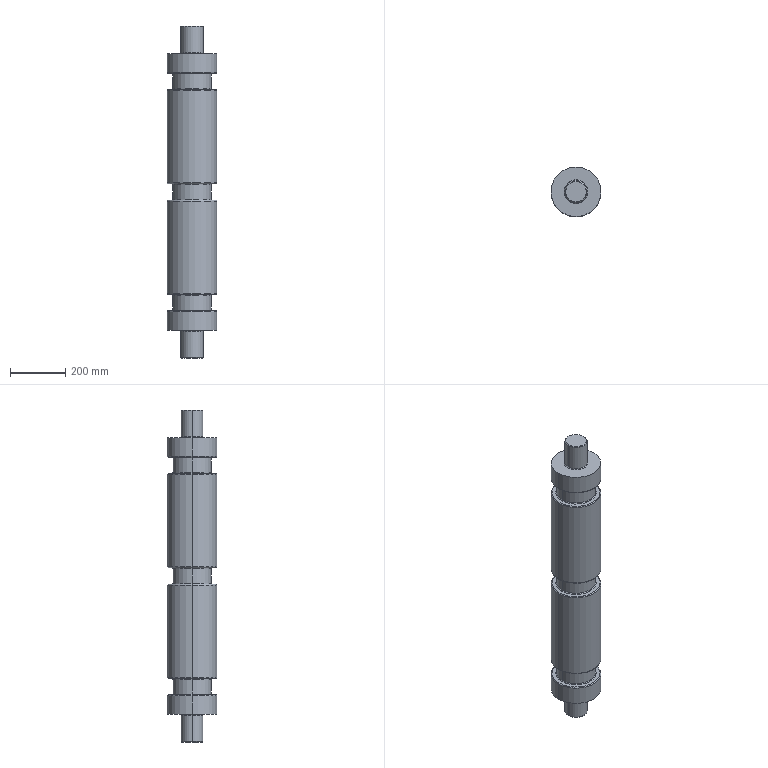Part | SolidWorks | features Chamfer 2, ICE 2, Extrusion 1, Fillet 1, LPattern 1, RefAxis 1, RevCut 1 | 1 solid | 60 faces | box 180 x 180 x 1200 mm | volume 24641407 mm3 | torus 24 | cylinder 18 | plane 10 | cone 8 | commonest cylinder face diameters 180 x8 140 x6 80 x4
STEP:
#1=CARTESIAN_POINT('',(-37.,0.,-100.));
#2=VERTEX_POINT('',#1);
#3=CARTESIAN_POINT('',(37.,0.,-100.));
#4=VERTEX_POINT('',#3);
#5=CARTESIAN_POINT('',(0.,0.,-100.));
#6=DIRECTION('',(0.,0.,-1.));
#7=DIRECTION('',(-1.,0.,0.));
#8=AXIS2_PLACEMENT_3D('',#5,#6,#7);
#9=CIRCLE('',#8,37.);
#10=EDGE_CURVE('',#2,#4,#9,.T.);
#11=ORIENTED_EDGE('',*,*,#10,.F.);
#12=CARTESIAN_POINT('',(-40.,0.,-97.));
#13=VERTEX_POINT('',#12);
#14=CARTESIAN_POINT('',(-37.,0.,-100.));
#15=DIRECTION('',(-0.7071,0.,0.7071));
#16=VECTOR('',#15,1000.);
#17=LINE('',#14,#16);
#18=EDGE_CURVE('',#2,#13,#17,.T.);
#19=ORIENTED_EDGE('',*,*,#18,.T.);
#20=CARTESIAN_POINT('',(40.,0.,-97.));
#21=VERTEX_POINT('',#20);
#22=CARTESIAN_POINT('',(0.,0.,-97.));
#23=DIRECTION('',(0.,0.,1.));
#24=DIRECTION('',(-1.,0.,0.));
#25=AXIS2_PLACEMENT_3D('',#22,#23,#24);
#26=CIRCLE('',#25,40.);
#27=EDGE_CURVE('',#21,#13,#26,.T.);
#28=ORIENTED_EDGE('',*,*,#27,.F.);
#29=CARTESIAN_POINT('',(37.,0.,-100.));
#30=DIRECTION('',(0.7071,0.,0.7071));
#31=VECTOR('',#30,1000.);
#32=LINE('',#29,#31);
#33=EDGE_CURVE('',#4,#21,#32,.T.);
#34=ORIENTED_EDGE('',*,*,#33,.F.);
#35=EDGE_LOOP('',(#11,#19,#28,#34));
#36=FACE_OUTER_BOUND('',#35,.T.);
#37=CARTESIAN_POINT('',(0.,0.,-100.));
#38=DIRECTION('',(0.,0.,1.));
#39=DIRECTION('',(1.,0.,0.));
#40=AXIS2_PLACEMENT_3D('',#37,#38,#39);
#41=CONICAL_SURFACE('',#40,37.,0.7854);
#42=ADVANCED_FACE('',(#36),#41,.T.);
#43=CARTESIAN_POINT('',(-40.,0.,-3.));
#44=VERTEX_POINT('',#43);
#45=CARTESIAN_POINT('',(40.,0.,-3.));
#46=VERTEX_POINT('',#45);
#47=CARTESIAN_POINT('',(0.,0.,-3.));
#48=DIRECTION('',(0.,0.,-1.));
#49=DIRECTION('',(1.,0.,0.));
#50=AXIS2_PLACEMENT_3D('',#47,#48,#49);
#51=CIRCLE('',#50,40.);
#52=EDGE_CURVE('',#44,#46,#51,.T.);
#53=ORIENTED_EDGE('',*,*,#52,.F.);
#54=CARTESIAN_POINT('',(-43.,0.,0.));
#55=VERTEX_POINT('',#54);
#56=CARTESIAN_POINT('',(-40.,0.,-3.));
#57=DIRECTION('',(-0.7071,0.,0.7071));
#58=VECTOR('',#57,1000.);
#59=LINE('',#56,#58);
#60=EDGE_CURVE('',#44,#55,#59,.T.);
#61=ORIENTED_EDGE('',*,*,#60,.T.);
#62=CARTESIAN_POINT('',(43.,0.,0.));
#63=VERTEX_POINT('',#62);
#64=CARTESIAN_POINT('',(0.,0.,0.));
#65=DIRECTION('',(0.,0.,1.));
#66=DIRECTION('',(1.,0.,0.));
#67=AXIS2_PLACEMENT_3D('',#64,#65,#66);
#68=CIRCLE('',#67,43.);
#69=EDGE_CURVE('',#63,#55,#68,.T.);
#70=ORIENTED_EDGE('',*,*,#69,.F.);
#71=CARTESIAN_POINT('',(40.,0.,-3.));
#72=DIRECTION('',(0.7071,0.,0.7071));
#73=VECTOR('',#72,1000.);
#74=LINE('',#71,#73);
#75=EDGE_CURVE('',#46,#63,#74,.T.);
#76=ORIENTED_EDGE('',*,*,#75,.F.);
#77=EDGE_LOOP('',(#53,#61,#70,#76));
#78=FACE_OUTER_BOUND('',#77,.T.);
#79=CARTESIAN_POINT('',(0.,0.,-3.));
#80=DIRECTION('',(0.,0.,1.));
#81=DIRECTION('',(1.,0.,0.));
#82=AXIS2_PLACEMENT_3D('',#79,#80,#81);
#83=CONICAL_SURFACE('',#82,40.,0.7854);
#84=ADVANCED_FACE('',(#78),#83,.T.);
#85=ORIENTED_EDGE('',*,*,#27,.T.);
#86=CARTESIAN_POINT('',(-40.,0.,-100.));
#87=DIRECTION('',(0.,0.,1.));
#88=VECTOR('',#87,1000.);
#89=LINE('',#86,#88);
#90=EDGE_CURVE('',#13,#44,#89,.T.);
#91=ORIENTED_EDGE('',*,*,#90,.T.);
#92=ORIENTED_EDGE('',*,*,#52,.T.);
#93=CARTESIAN_POINT('',(40.,0.,-100.));
#94=DIRECTION('',(0.,0.,1.));
#95=VECTOR('',#94,1000.);
#96=LINE('',#93,#95);
#97=EDGE_CURVE('',#21,#46,#96,.T.);
#98=ORIENTED_EDGE('',*,*,#97,.F.);
#99=EDGE_LOOP('',(#85,#91,#92,#98));
#100=FACE_OUTER_BOUND('',#99,.T.);
#101=CARTESIAN_POINT('',(0.,0.,-100.));
#102=DIRECTION('',(0.,0.,1.));
#103=DIRECTION('',(1.,0.,0.));
#104=AXIS2_PLACEMENT_3D('',#101,#102,#103);
#105=CYLINDRICAL_SURFACE('',#104,40.);
#106=ADVANCED_FACE('',(#100),#105,.T.);
#107=CARTESIAN_POINT('',(37.,0.,1100.));
#108=VERTEX_POINT('',#107);
#109=CARTESIAN_POINT('',(-37.,0.,1100.));
#110=VERTEX_POINT('',#109);
#111=CARTESIAN_POINT('',(0.,0.,1100.));
#112=DIRECTION('',(0.,0.,1.));
#113=DIRECTION('',(1.,0.,0.));
#114=AXIS2_PLACEMENT_3D('',#111,#112,#113);
#115=CIRCLE('',#114,37.);
#116=EDGE_CURVE('',#108,#110,#115,.T.);
#117=ORIENTED_EDGE('',*,*,#116,.F.);
#118=CARTESIAN_POINT('',(40.,0.,1097.));
#119=VERTEX_POINT('',#118);
#120=CARTESIAN_POINT('',(37.,0.,1100.));
#121=DIRECTION('',(0.7071,0.,-0.7071));
#122=VECTOR('',#121,1000.);
#123=LINE('',#120,#122);
#124=EDGE_CURVE('',#108,#119,#123,.T.);
#125=ORIENTED_EDGE('',*,*,#124,.T.);
#126=CARTESIAN_POINT('',(-40.,0.,1097.));
#127=VERTEX_POINT('',#126);
#128=CARTESIAN_POINT('',(0.,0.,1097.));
#129=DIRECTION('',(0.,0.,-1.));
#130=DIRECTION('',(1.,0.,0.));
#131=AXIS2_PLACEMENT_3D('',#128,#129,#130);
#132=CIRCLE('',#131,40.);
#133=EDGE_CURVE('',#127,#119,#132,.T.);
#134=ORIENTED_EDGE('',*,*,#133,.F.);
#135=CARTESIAN_POINT('',(-37.,0.,1100.));
#136=DIRECTION('',(-0.7071,0.,-0.7071));
#137=VECTOR('',#136,1000.);
#138=LINE('',#135,#137);
#139=EDGE_CURVE('',#110,#127,#138,.T.);
#140=ORIENTED_EDGE('',*,*,#139,.F.);
#141=EDGE_LOOP('',(#117,#125,#134,#140));
#142=FACE_OUTER_BOUND('',#141,.T.);
#143=CARTESIAN_POINT('',(0.,0.,1100.));
#144=DIRECTION('',(0.,0.,-1.));
#145=DIRECTION('',(-1.,0.,0.));
#146=AXIS2_PLACEMENT_3D('',#143,#144,#145);
#147=CONICAL_SURFACE('',#146,37.,0.7854);
#148=ADVANCED_FACE('',(#142),#147,.T.);
#149=CARTESIAN_POINT('',(40.,0.,1003.));
#150=VERTEX_POINT('',#149);
#151=CARTESIAN_POINT('',(-40.,0.,1003.));
#152=VERTEX_POINT('',#151);
#153=CARTESIAN_POINT('',(0.,0.,1003.));
#154=DIRECTION('',(0.,0.,1.));
#155=DIRECTION('',(1.,0.,0.));
#156=AXIS2_PLACEMENT_3D('',#153,#154,#155);
#157=CIRCLE('',#156,40.);
#158=EDGE_CURVE('',#150,#152,#157,.T.);
#159=ORIENTED_EDGE('',*,*,#158,.F.);
#160=CARTESIAN_POINT('',(43.,0.,1000.));
#161=VERTEX_POINT('',#160);
#162=CARTESIAN_POINT('',(40.,0.,1003.));
#163=DIRECTION('',(0.7071,0.,-0.7071));
#164=VECTOR('',#163,1000.);
#165=LINE('',#162,#164);
#166=EDGE_CURVE('',#150,#161,#165,.T.);
#167=ORIENTED_EDGE('',*,*,#166,.T.);
#168=CARTESIAN_POINT('',(-43.,0.,1000.));
#169=VERTEX_POINT('',#168);
#170=CARTESIAN_POINT('',(0.,0.,1000.));
#171=DIRECTION('',(0.,0.,-1.));
#172=DIRECTION('',(1.,0.,0.));
#173=AXIS2_PLACEMENT_3D('',#170,#171,#172);
#174=CIRCLE('',#173,43.);
#175=EDGE_CURVE('',#169,#161,#174,.T.);
#176=ORIENTED_EDGE('',*,*,#175,.F.);
#177=CARTESIAN_POINT('',(-40.,0.,1003.));
#178=DIRECTION('',(-0.7071,0.,-0.7071));
#179=VECTOR('',#178,1000.);
#180=LINE('',#177,#179);
#181=EDGE_CURVE('',#152,#169,#180,.T.);
#182=ORIENTED_EDGE('',*,*,#181,.F.);
#183=EDGE_LOOP('',(#159,#167,#176,#182));
#184=FACE_OUTER_BOUND('',#183,.T.);
#185=CARTESIAN_POINT('',(0.,0.,1003.));
#186=DIRECTION('',(0.,0.,-1.));
#187=DIRECTION('',(-1.,0.,0.));
#188=AXIS2_PLACEMENT_3D('',#185,#186,#187);
#189=CONICAL_SURFACE('',#188,40.,0.7854);
#190=ADVANCED_FACE('',(#184),#189,.T.);
#191=ORIENTED_EDGE('',*,*,#133,.T.);
#192=CARTESIAN_POINT('',(40.,0.,1100.));
#193=DIRECTION('',(0.,0.,-1.));
#194=VECTOR('',#193,1000.);
#195=LINE('',#192,#194);
#196=EDGE_CURVE('',#119,#150,#195,.T.);
#197=ORIENTED_EDGE('',*,*,#196,.T.);
#198=ORIENTED_EDGE('',*,*,#158,.T.);
#199=CARTESIAN_POINT('',(-40.,0.,1100.));
#200=DIRECTION('',(0.,0.,-1.));
#201=VECTOR('',#200,1000.);
#202=LINE('',#199,#201);
#203=EDGE_CURVE('',#127,#152,#202,.T.);
#204=ORIENTED_EDGE('',*,*,#203,.F.);
#205=EDGE_LOOP('',(#191,#197,#198,#204));
#206=FACE_OUTER_BOUND('',#205,.T.);
#207=CARTESIAN_POINT('',(0.,0.,1100.));
#208=DIRECTION('',(0.,0.,-1.));
#209=DIRECTION('',(-1.,0.,0.));
#210=AXIS2_PLACEMENT_3D('',#207,#208,#209);
#211=CYLINDRICAL_SURFACE('',#210,40.);
#212=ADVANCED_FACE('',(#206),#211,.T.);
#213=CARTESIAN_POINT('',(-70.,0.,73.));
#214=VERTEX_POINT('',#213);
#215=CARTESIAN_POINT('',(70.,0.,73.));
#216=VERTEX_POINT('',#215);
#217=CARTESIAN_POINT('',(0.,0.,73.));
#218=DIRECTION('',(0.,0.,1.));
#219=DIRECTION('',(1.,0.,0.));
#220=AXIS2_PLACEMENT_3D('',#217,#218,#219);
#221=CIRCLE('',#220,70.);
#222=EDGE_CURVE('',#214,#216,#221,.T.);
#223=ORIENTED_EDGE('',*,*,#222,.F.);
#224=CARTESIAN_POINT('',(-73.,0.,70.));
#225=VERTEX_POINT('',#224);
#226=CARTESIAN_POINT('',(-73.,0.,73.));
#227=DIRECTION('',(0.,1.,0.));
#228=DIRECTION('',(-1.,0.,0.));
#229=AXIS2_PLACEMENT_3D('',#226,#227,#228);
#230=CIRCLE('',#229,3.);
#231=EDGE_CURVE('',#214,#225,#230,.T.);
#232=ORIENTED_EDGE('',*,*,#231,.T.);
#233=CARTESIAN_POINT('',(73.,0.,70.));
#234=VERTEX_POINT('',#233);
#235=CARTESIAN_POINT('',(0.,0.,70.));
#236=DIRECTION('',(0.,0.,-1.));
#237=DIRECTION('',(1.,0.,0.));
#238=AXIS2_PLACEMENT_3D('',#235,#236,#237);
#239=CIRCLE('',#238,73.);
#240=EDGE_CURVE('',#234,#225,#239,.T.);
#241=ORIENTED_EDGE('',*,*,#240,.F.);
#242=CARTESIAN_POINT('',(73.,0.,73.));
#243=DIRECTION('',(0.,-1.,0.));
#244=DIRECTION('',(0.,0.,-1.));
#245=AXIS2_PLACEMENT_3D('',#242,#243,#244);
#246=CIRCLE('',#245,3.);
#247=EDGE_CURVE('',#216,#234,#246,.T.);
#248=ORIENTED_EDGE('',*,*,#247,.F.);
#249=EDGE_LOOP('',(#223,#232,#241,#248));
#250=FACE_OUTER_BOUND('',#249,.T.);
#251=CARTESIAN_POINT('',(0.,0.,73.));
#252=DIRECTION('',(0.,0.,1.));
#253=DIRECTION('',(1.,0.,0.));
#254=AXIS2_PLACEMENT_3D('',#251,#252,#253);
#255=TOROIDAL_SURFACE('',#254,73.,3.);
#256=ADVANCED_FACE('',(#250),#255,.F.);
#257=CARTESIAN_POINT('',(-90.,0.,67.));
#258=VERTEX_POINT('',#257);
#259=CARTESIAN_POINT('',(90.,0.,67.));
#260=VERTEX_POINT('',#259);
#261=CARTESIAN_POINT('',(0.,0.,67.));
#262=DIRECTION('',(0.,0.,-1.));
#263=DIRECTION('',(1.,0.,0.));
#264=AXIS2_PLACEMENT_3D('',#261,#262,#263);
#265=CIRCLE('',#264,90.);
#266=EDGE_CURVE('',#258,#260,#265,.T.);
#267=ORIENTED_EDGE('',*,*,#266,.F.);
#268=CARTESIAN_POINT('',(-87.,0.,70.));
#269=VERTEX_POINT('',#268);
#270=CARTESIAN_POINT('',(-87.,0.,67.));
#271=DIRECTION('',(0.,1.,0.));
#272=DIRECTION('',(-1.,0.,0.));
#273=AXIS2_PLACEMENT_3D('',#270,#271,#272);
#274=CIRCLE('',#273,3.);
#275=EDGE_CURVE('',#258,#269,#274,.T.);
#276=ORIENTED_EDGE('',*,*,#275,.T.);
#277=CARTESIAN_POINT('',(87.,0.,70.));
#278=VERTEX_POINT('',#277);
#279=CARTESIAN_POINT('',(0.,0.,70.));
#280=DIRECTION('',(0.,0.,1.));
#281=DIRECTION('',(1.,0.,0.));
#282=AXIS2_PLACEMENT_3D('',#279,#280,#281);
#283=CIRCLE('',#282,87.);
#284=EDGE_CURVE('',#278,#269,#283,.T.);
#285=ORIENTED_EDGE('',*,*,#284,.F.);
#286=CARTESIAN_POINT('',(87.,0.,67.));
#287=DIRECTION('',(0.,-1.,0.));
#288=DIRECTION('',(0.,0.,-1.));
#289=AXIS2_PLACEMENT_3D('',#286,#287,#288);
#290=CIRCLE('',#289,3.);
#291=EDGE_CURVE('',#260,#278,#290,.T.);
#292=ORIENTED_EDGE('',*,*,#291,.F.);
#293=EDGE_LOOP('',(#267,#276,#285,#292));
#294=FACE_OUTER_BOUND('',#293,.T.);
#295=CARTESIAN_POINT('',(0.,0.,67.));
#296=DIRECTION('',(0.,0.,1.));
#297=DIRECTION('',(1.,0.,0.));
#298=AXIS2_PLACEMENT_3D('',#295,#296,#297);
#299=TOROIDAL_SURFACE('',#298,87.,3.);
#300=ADVANCED_FACE('',(#294),#299,.T.);
#301=CARTESIAN_POINT('',(90.,0.,133.));
#302=VERTEX_POINT('',#301);
#303=CARTESIAN_POINT('',(-90.,0.,133.));
#304=VERTEX_POINT('',#303);
#305=CARTESIAN_POINT('',(0.,0.,133.));
#306=DIRECTION('',(0.,0.,1.));
#307=DIRECTION('',(-1.,0.,0.));
#308=AXIS2_PLACEMENT_3D('',#305,#306,#307);
#309=CIRCLE('',#308,90.);
#310=EDGE_CURVE('',#302,#304,#309,.T.);
#311=ORIENTED_EDGE('',*,*,#310,.F.);
#312=CARTESIAN_POINT('',(87.,0.,130.));
#313=VERTEX_POINT('',#312);
#314=CARTESIAN_POINT('',(87.,0.,133.));
#315=DIRECTION('',(0.,1.,0.));
#316=DIRECTION('',(-1.,0.,0.));
#317=AXIS2_PLACEMENT_3D('',#314,#315,#316);
#318=CIRCLE('',#317,3.);
#319=EDGE_CURVE('',#302,#313,#318,.T.);
#320=ORIENTED_EDGE('',*,*,#319,.T.);
#321=CARTESIAN_POINT('',(-87.,0.,130.));
#322=VERTEX_POINT('',#321);
#323=CARTESIAN_POINT('',(0.,0.,130.));
#324=DIRECTION('',(0.,0.,-1.));
#325=DIRECTION('',(-1.,0.,0.));
#326=AXIS2_PLACEMENT_3D('',#323,#324,#325);
#327=CIRCLE('',#326,87.);
#328=EDGE_CURVE('',#322,#313,#327,.T.);
#329=ORIENTED_EDGE('',*,*,#328,.F.);
#330=CARTESIAN_POINT('',(-87.,0.,133.));
#331=DIRECTION('',(0.,-1.,0.));
#332=DIRECTION('',(0.,0.,-1.));
#333=AXIS2_PLACEMENT_3D('',#330,#331,#332);
#334=CIRCLE('',#333,3.);
#335=EDGE_CURVE('',#304,#322,#334,.T.);
#336=ORIENTED_EDGE('',*,*,#335,.F.);
#337=EDGE_LOOP('',(#311,#320,#329,#336));
#338=FACE_OUTER_BOUND('',#337,.T.);
#339=CARTESIAN_POINT('',(0.,0.,133.));
#340=DIRECTION('',(0.,0.,-1.));
#341=DIRECTION('',(-1.,0.,0.));
#342=AXIS2_PLACEMENT_3D('',#339,#340,#341);
#343=TOROIDAL_SURFACE('',#342,87.,3.);
#344=ADVANCED_FACE('',(#338),#343,.T.);
#345=CARTESIAN_POINT('',(70.,0.,127.));
#346=VERTEX_POINT('',#345);
#347=CARTESIAN_POINT('',(-70.,0.,127.));
#348=VERTEX_POINT('',#347);
#349=CARTESIAN_POINT('',(0.,0.,127.));
#350=DIRECTION('',(0.,0.,-1.));
#351=DIRECTION('',(-1.,0.,0.));
#352=AXIS2_PLACEMENT_3D('',#349,#350,#351);
#353=CIRCLE('',#352,70.);
#354=EDGE_CURVE('',#346,#348,#353,.T.);
#355=ORIENTED_EDGE('',*,*,#354,.F.);
#356=CARTESIAN_POINT('',(73.,0.,130.));
#357=VERTEX_POINT('',#356);
#358=CARTESIAN_POINT('',(73.,0.,127.));
#359=DIRECTION('',(0.,1.,0.));
#360=DIRECTION('',(-1.,0.,0.));
#361=AXIS2_PLACEMENT_3D('',#358,#359,#360);
#362=CIRCLE('',#361,3.);
#363=EDGE_CURVE('',#346,#357,#362,.T.);
#364=ORIENTED_EDGE('',*,*,#363,.T.);
#365=CARTESIAN_POINT('',(-73.,0.,130.));
#366=VERTEX_POINT('',#365);
#367=CARTESIAN_POINT('',(0.,0.,130.));
#368=DIRECTION('',(0.,0.,1.));
#369=DIRECTION('',(-1.,0.,0.));
#370=AXIS2_PLACEMENT_3D('',#367,#368,#369);
#371=CIRCLE('',#370,73.);
#372=EDGE_CURVE('',#366,#357,#371,.T.);
#373=ORIENTED_EDGE('',*,*,#372,.F.);
#374=CARTESIAN_POINT('',(-73.,0.,127.));
#375=DIRECTION('',(0.,-1.,0.));
#376=DIRECTION('',(0.,0.,-1.));
#377=AXIS2_PLACEMENT_3D('',#374,#375,#376);
#378=CIRCLE('',#377,3.);
#379=EDGE_CURVE('',#348,#366,#378,.T.);
#380=ORIENTED_EDGE('',*,*,#379,.F.);
#381=EDGE_LOOP('',(#355,#364,#373,#380));
#382=FACE_OUTER_BOUND('',#381,.T.);
#383=CARTESIAN_POINT('',(0.,0.,127.));
#384=DIRECTION('',(0.,0.,-1.));
#385=DIRECTION('',(-1.,0.,0.));
#386=AXIS2_PLACEMENT_3D('',#383,#384,#385);
#387=TOROIDAL_SURFACE('',#386,73.,3.);
#388=ADVANCED_FACE('',(#382),#387,.F.);
#389=CARTESIAN_POINT('',(-70.,0.,873.));
#390=VERTEX_POINT('',#389);
#391=CARTESIAN_POINT('',(70.,0.,873.));
#392=VERTEX_POINT('',#391);
#393=CARTESIAN_POINT('',(0.,0.,873.));
#394=DIRECTION('',(0.,0.,1.));
#395=DIRECTION('',(1.,0.,0.));
#396=AXIS2_PLACEMENT_3D('',#393,#394,#395);
#397=CIRCLE('',#396,70.);
#398=EDGE_CURVE('',#390,#392,#397,.T.);
#399=ORIENTED_EDGE('',*,*,#398,.F.);
#400=CARTESIAN_POINT('',(-73.,0.,870.));
#401=VERTEX_POINT('',#400);
#402=CARTESIAN_POINT('',(-73.,0.,873.));
#403=DIRECTION('',(0.,1.,0.));
#404=DIRECTION('',(-1.,0.,0.));
#405=AXIS2_PLACEMENT_3D('',#402,#403,#404);
#406=CIRCLE('',#405,3.);
#407=EDGE_CURVE('',#390,#401,#406,.T.);
#408=ORIENTED_EDGE('',*,*,#407,.T.);
#409=CARTESIAN_POINT('',(73.,0.,870.));
#410=VERTEX_POINT('',#409);
#411=CARTESIAN_POINT('',(0.,0.,870.));
#412=DIRECTION('',(0.,0.,-1.));
#413=DIRECTION('',(1.,0.,0.));
#414=AXIS2_PLACEMENT_3D('',#411,#412,#413);
#415=CIRCLE('',#414,73.);
#416=EDGE_CURVE('',#410,#401,#415,.T.);
#417=ORIENTED_EDGE('',*,*,#416,.F.);
#418=CARTESIAN_POINT('',(73.,0.,873.));
#419=DIRECTION('',(0.,-1.,0.));
#420=DIRECTION('',(0.,0.,-1.));
#421=AXIS2_PLACEMENT_3D('',#418,#419,#420);
#422=CIRCLE('',#421,3.);
#423=EDGE_CURVE('',#392,#410,#422,.T.);
#424=ORIENTED_EDGE('',*,*,#423,.F.);
#425=EDGE_LOOP('',(#399,#408,#417,#424));
#426=FACE_OUTER_BOUND('',#425,.T.);
#427=CARTESIAN_POINT('',(0.,0.,873.));
#428=DIRECTION('',(0.,0.,1.));
#429=DIRECTION('',(1.,0.,0.));
#430=AXIS2_PLACEMENT_3D('',#427,#428,#429);
#431=TOROIDAL_SURFACE('',#430,73.,3.);
#432=ADVANCED_FACE('',(#426),#431,.F.);
#433=CARTESIAN_POINT('',(-90.,0.,867.));
#434=VERTEX_POINT('',#433);
#435=CARTESIAN_POINT('',(90.,0.,867.));
#436=VERTEX_POINT('',#435);
#437=CARTESIAN_POINT('',(0.,0.,867.));
#438=DIRECTION('',(0.,0.,-1.));
#439=DIRECTION('',(1.,0.,0.));
#440=AXIS2_PLACEMENT_3D('',#437,#438,#439);
#441=CIRCLE('',#440,90.);
#442=EDGE_CURVE('',#434,#436,#441,.T.);
#443=ORIENTED_EDGE('',*,*,#442,.F.);
#444=CARTESIAN_POINT('',(-87.,0.,870.));
#445=VERTEX_POINT('',#444);
#446=CARTESIAN_POINT('',(-87.,0.,867.));
#447=DIRECTION('',(0.,1.,0.));
#448=DIRECTION('',(-1.,0.,0.));
#449=AXIS2_PLACEMENT_3D('',#446,#447,#448);
#450=CIRCLE('',#449,3.);
#451=EDGE_CURVE('',#434,#445,#450,.T.);
#452=ORIENTED_EDGE('',*,*,#451,.T.);
#453=CARTESIAN_POINT('',(87.,0.,870.));
#454=VERTEX_POINT('',#453);
#455=CARTESIAN_POINT('',(0.,0.,870.));
#456=DIRECTION('',(0.,0.,1.));
#457=DIRECTION('',(1.,0.,0.));
#458=AXIS2_PLACEMENT_3D('',#455,#456,#457);
#459=CIRCLE('',#458,87.);
#460=EDGE_CURVE('',#454,#445,#459,.T.);
#461=ORIENTED_EDGE('',*,*,#460,.F.);
#462=CARTESIAN_POINT('',(87.,0.,867.));
#463=DIRECTION('',(0.,-1.,0.));
#464=DIRECTION('',(0.,0.,-1.));
#465=AXIS2_PLACEMENT_3D('',#462,#463,#464);
#466=CIRCLE('',#465,3.);
#467=EDGE_CURVE('',#436,#454,#466,.T.);
#468=ORIENTED_EDGE('',*,*,#467,.F.);
#469=EDGE_LOOP('',(#443,#452,#461,#468));
#470=FACE_OUTER_BOUND('',#469,.T.);
#471=CARTESIAN_POINT('',(0.,0.,867.));
#472=DIRECTION('',(0.,0.,1.));
#473=DIRECTION('',(1.,0.,0.));
#474=AXIS2_PLACEMENT_3D('',#471,#472,#473);
#475=TOROIDAL_SURFACE('',#474,87.,3.);
#476=ADVANCED_FACE('',(#470),#475,.T.);
#477=CARTESIAN_POINT('',(90.,0.,933.));
#478=VERTEX_POINT('',#477);
#479=CARTESIAN_POINT('',(-90.,0.,933.));
#480=VERTEX_POINT('',#479);
#481=CARTESIAN_POINT('',(0.,0.,933.));
#482=DIRECTION('',(0.,0.,1.));
#483=DIRECTION('',(-1.,0.,0.));
#484=AXIS2_PLACEMENT_3D('',#481,#482,#483);
#485=CIRCLE('',#484,90.);
#486=EDGE_CURVE('',#478,#480,#485,.T.);
#487=ORIENTED_EDGE('',*,*,#486,.F.);
#488=CARTESIAN_POINT('',(87.,0.,930.));
#489=VERTEX_POINT('',#488);
#490=CARTESIAN_POINT('',(87.,0.,933.));
#491=DIRECTION('',(0.,1.,0.));
#492=DIRECTION('',(-1.,0.,0.));
#493=AXIS2_PLACEMENT_3D('',#490,#491,#492);
#494=CIRCLE('',#493,3.);
#495=EDGE_CURVE('',#478,#489,#494,.T.);
#496=ORIENTED_EDGE('',*,*,#495,.T.);
#497=CARTESIAN_POINT('',(-87.,0.,930.));
#498=VERTEX_POINT('',#497);
#499=CARTESIAN_POINT('',(0.,0.,930.));
#500=DIRECTION('',(0.,0.,-1.));
#501=DIRECTION('',(-1.,0.,0.));
#502=AXIS2_PLACEMENT_3D('',#499,#500,#501);
#503=CIRCLE('',#502,87.);
#504=EDGE_CURVE('',#498,#489,#503,.T.);
#505=ORIENTED_EDGE('',*,*,#504,.F.);
#506=CARTESIAN_POINT('',(-87.,0.,933.));
#507=DIRECTION('',(0.,-1.,0.));
#508=DIRECTION('',(0.,0.,-1.));
#509=AXIS2_PLACEMENT_3D('',#506,#507,#508);
#510=CIRCLE('',#509,3.);
#511=EDGE_CURVE('',#480,#498,#510,.T.);
#512=ORIENTED_EDGE('',*,*,#511,.F.);
#513=EDGE_LOOP('',(#487,#496,#505,#512));
#514=FACE_OUTER_BOUND('',#513,.T.);
#515=CARTESIAN_POINT('',(0.,0.,933.));
#516=DIRECTION('',(0.,0.,-1.));
#517=DIRECTION('',(-1.,0.,0.));
#518=AXIS2_PLACEMENT_3D('',#515,#516,#517);
#519=TOROIDAL_SURFACE('',#518,87.,3.);
#520=ADVANCED_FACE('',(#514),#519,.T.);
#521=CARTESIAN_POINT('',(70.,0.,927.));
#522=VERTEX_POINT('',#521);
#523=CARTESIAN_POINT('',(-70.,0.,927.));
#524=VERTEX_POINT('',#523);
#525=CARTESIAN_POINT('',(0.,0.,927.));
#526=DIRECTION('',(0.,0.,-1.));
#527=DIRECTION('',(-1.,0.,0.));
#528=AXIS2_PLACEMENT_3D('',#525,#526,#527);
#529=CIRCLE('',#528,70.);
#530=EDGE_CURVE('',#522,#524,#529,.T.);
#531=ORIENTED_EDGE('',*,*,#530,.F.);
#532=CARTESIAN_POINT('',(73.,0.,930.));
#533=VERTEX_POINT('',#532);
#534=CARTESIAN_POINT('',(73.,0.,927.));
#535=DIRECTION('',(0.,1.,0.));
#536=DIRECTION('',(-1.,0.,0.));
#537=AXIS2_PLACEMENT_3D('',#534,#535,#536);
#538=CIRCLE('',#537,3.);
#539=EDGE_CURVE('',#522,#533,#538,.T.);
#540=ORIENTED_EDGE('',*,*,#539,.T.);
#541=CARTESIAN_POINT('',(-73.,0.,930.));
#542=VERTEX_POINT('',#541);
#543=CARTESIAN_POINT('',(0.,0.,930.));
#544=DIRECTION('',(0.,0.,1.));
#545=DIRECTION('',(-1.,0.,0.));
#546=AXIS2_PLACEMENT_3D('',#543,#544,#545);
#547=CIRCLE('',#546,73.);
#548=EDGE_CURVE('',#542,#533,#547,.T.);
#549=ORIENTED_EDGE('',*,*,#548,.F.);
#550=CARTESIAN_POINT('',(-73.,0.,927.));
#551=DIRECTION('',(0.,-1.,0.));
#552=DIRECTION('',(0.,0.,-1.));
#553=AXIS2_PLACEMENT_3D('',#550,#551,#552);
#554=CIRCLE('',#553,3.);
#555=EDGE_CURVE('',#524,#542,#554,.T.);
#556=ORIENTED_EDGE('',*,*,#555,.F.);
#557=EDGE_LOOP('',(#531,#540,#549,#556));
#558=FACE_OUTER_BOUND('',#557,.T.);
#559=CARTESIAN_POINT('',(0.,0.,927.));
#560=DIRECTION('',(0.,0.,-1.));
#561=DIRECTION('',(-1.,0.,0.));
#562=AXIS2_PLACEMENT_3D('',#559,#560,#561);
#563=TOROIDAL_SURFACE('',#562,73.,3.);
#564=ADVANCED_FACE('',(#558),#563,.F.);
#565=ORIENTED_EDGE('',*,*,#266,.T.);
#566=CARTESIAN_POINT('',(90.,0.,0.));
#567=VERTEX_POINT('',#566);
#568=CARTESIAN_POINT('',(90.,0.,1000.));
#569=DIRECTION('',(0.,0.,-1.));
#570=VECTOR('',#569,1000.);
#571=LINE('',#568,#570);
#572=EDGE_CURVE('',#260,#567,#571,.T.);
#573=ORIENTED_EDGE('',*,*,#572,.T.);
#574=CARTESIAN_POINT('',(-90.,0.,0.));
#575=VERTEX_POINT('',#574);
#576=CARTESIAN_POINT('',(0.,0.,0.));
#577=DIRECTION('',(0.,0.,1.));
#578=DIRECTION('',(1.,0.,0.));
#579=AXIS2_PLACEMENT_3D('',#576,#577,#578);
#580=CIRCLE('',#579,90.);
#581=EDGE_CURVE('',#567,#575,#580,.T.);
#582=ORIENTED_EDGE('',*,*,#581,.T.);
#583=CARTESIAN_POINT('',(-90.,0.,1000.));
#584=DIRECTION('',(0.,0.,-1.));
#585=VECTOR('',#584,1000.);
#586=LINE('',#583,#585);
#587=EDGE_CURVE('',#258,#575,#586,.T.);
#588=ORIENTED_EDGE('',*,*,#587,.F.);
#589=EDGE_LOOP('',(#565,#573,#582,#588));
#590=FACE_OUTER_BOUND('',#589,.T.);
#591=CARTESIAN_POINT('',(0.,0.,1000.));
#592=DIRECTION('',(0.,0.,-1.));
#593=DIRECTION('',(-1.,0.,0.));
#594=AXIS2_PLACEMENT_3D('',#591,#592,#593);
#595=CYLINDRICAL_SURFACE('',#594,90.);
#596=ADVANCED_FACE('',(#590),#595,.T.);
#597=CARTESIAN_POINT('',(0.,0.,127.));
#598=DIRECTION('',(0.,0.,-1.));
#599=DIRECTION('',(-1.,0.,0.));
#600=AXIS2_PLACEMENT_3D('',#597,#598,#599);
#601=CIRCLE('',#600,70.);
#602=EDGE_CURVE('',#348,#346,#601,.T.);
#603=ORIENTED_EDGE('',*,*,#602,.T.);
#604=CARTESIAN_POINT('',(70.,0.,-400.));
#605=DIRECTION('',(0.,0.,-1.));
#606=VECTOR('',#605,1000.);
#607=LINE('',#604,#606);
#608=EDGE_CURVE('',#346,#216,#607,.T.);
#609=ORIENTED_EDGE('',*,*,#608,.T.);
#610=CARTESIAN_POINT('',(0.,0.,73.));
#611=DIRECTION('',(0.,0.,1.));
#612=DIRECTION('',(1.,0.,0.));
#613=AXIS2_PLACEMENT_3D('',#610,#611,#612);
#614=CIRCLE('',#613,70.);
#615=EDGE_CURVE('',#216,#214,#614,.T.);
#616=ORIENTED_EDGE('',*,*,#615,.T.);
#617=CARTESIAN_POINT('',(-70.,0.,-400.));
#618=DIRECTION('',(0.,0.,-1.));
#619=VECTOR('',#618,1000.);
#620=LINE('',#617,#619);
#621=EDGE_CURVE('',#348,#214,#620,.T.);
#622=ORIENTED_EDGE('',*,*,#621,.F.);
#623=EDGE_LOOP('',(#603,#609,#616,#622));
#624=FACE_OUTER_BOUND('',#623,.T.);
#625=CARTESIAN_POINT('',(0.,0.,-400.));
#626=DIRECTION('',(0.,0.,-1.));
#627=DIRECTION('',(-1.,0.,0.));
#628=AXIS2_PLACEMENT_3D('',#625,#626,#627);
#629=CYLINDRICAL_SURFACE('',#628,70.);
#630=ADVANCED_FACE('',(#624),#629,.T.);
#631=CARTESIAN_POINT('',(90.,0.,1000.));
#632=VERTEX_POINT('',#631);
#633=CARTESIAN_POINT('',(-90.,0.,1000.));
#634=VERTEX_POINT('',#633);
#635=CARTESIAN_POINT('',(0.,0.,1000.));
#636=DIRECTION('',(0.,0.,1.));
#637=DIRECTION('',(1.,0.,0.));
#638=AXIS2_PLACEMENT_3D('',#635,#636,#637);
#639=CIRCLE('',#638,90.);
#640=EDGE_CURVE('',#632,#634,#639,.T.);
#641=ORIENTED_EDGE('',*,*,#640,.F.);
#642=CARTESIAN_POINT('',(90.,0.,1000.));
#643=DIRECTION('',(0.,0.,-1.));
#644=VECTOR('',#643,1000.);
#645=LINE('',#642,#644);
#646=EDGE_CURVE('',#632,#478,#645,.T.);
#647=ORIENTED_EDGE('',*,*,#646,.T.);
#648=ORIENTED_EDGE('',*,*,#486,.T.);
#649=CARTESIAN_POINT('',(-90.,0.,1000.));
#650=DIRECTION('',(0.,0.,-1.));
#651=VECTOR('',#650,1000.);
#652=LINE('',#649,#651);
#653=EDGE_CURVE('',#634,#480,#652,.T.);
#654=ORIENTED_EDGE('',*,*,#653,.F.);
#655=EDGE_LOOP('',(#641,#647,#648,#654));
#656=FACE_OUTER_BOUND('',#655,.T.);
#657=CARTESIAN_POINT('',(0.,0.,1000.));
#658=DIRECTION('',(0.,0.,-1.));
#659=DIRECTION('',(-1.,0.,0.));
#660=AXIS2_PLACEMENT_3D('',#657,#658,#659);
#661=CYLINDRICAL_SURFACE('',#660,90.);
#662=ADVANCED_FACE('',(#656),#661,.T.);
#663=CARTESIAN_POINT('',(0.,0.,927.));
#664=DIRECTION('',(0.,0.,-1.));
#665=DIRECTION('',(-1.,0.,0.));
#666=AXIS2_PLACEMENT_3D('',#663,#664,#665);
#667=CIRCLE('',#666,70.);
#668=EDGE_CURVE('',#524,#522,#667,.T.);
#669=ORIENTED_EDGE('',*,*,#668,.T.);
#670=CARTESIAN_POINT('',(70.,0.,400.));
#671=DIRECTION('',(0.,0.,-1.));
#672=VECTOR('',#671,1000.);
#673=LINE('',#670,#672);
#674=EDGE_CURVE('',#522,#392,#673,.T.);
#675=ORIENTED_EDGE('',*,*,#674,.T.);
#676=CARTESIAN_POINT('',(0.,0.,873.));
#677=DIRECTION('',(0.,0.,1.));
#678=DIRECTION('',(1.,0.,0.));
#679=AXIS2_PLACEMENT_3D('',#676,#677,#678);
#680=CIRCLE('',#679,70.);
#681=EDGE_CURVE('',#392,#390,#680,.T.);
#682=ORIENTED_EDGE('',*,*,#681,.T.);
#683=CARTESIAN_POINT('',(-70.,0.,400.));
#684=DIRECTION('',(0.,0.,-1.));
#685=VECTOR('',#684,1000.);
#686=LINE('',#683,#685);
#687=EDGE_CURVE('',#524,#390,#686,.T.);
#688=ORIENTED_EDGE('',*,*,#687,.F.);
#689=EDGE_LOOP('',(#669,#675,#682,#688));
#690=FACE_OUTER_BOUND('',#689,.T.);
#691=CARTESIAN_POINT('',(0.,0.,400.));
#692=DIRECTION('',(0.,0.,-1.));
#693=DIRECTION('',(-1.,0.,0.));
#694=AXIS2_PLACEMENT_3D('',#691,#692,#693);
#695=CYLINDRICAL_SURFACE('',#694,70.);
#696=ADVANCED_FACE('',(#690),#695,.T.);
#697=CARTESIAN_POINT('',(-70.,0.,473.));
#698=VERTEX_POINT('',#697);
#699=CARTESIAN_POINT('',(70.,0.,473.));
#700=VERTEX_POINT('',#699);
#701=CARTESIAN_POINT('',(0.,0.,473.));
#702=DIRECTION('',(0.,0.,1.));
#703=DIRECTION('',(1.,0.,0.));
#704=AXIS2_PLACEMENT_3D('',#701,#702,#703);
#705=CIRCLE('',#704,70.);
#706=EDGE_CURVE('',#698,#700,#705,.T.);
#707=ORIENTED_EDGE('',*,*,#706,.F.);
#708=CARTESIAN_POINT('',(-73.,0.,470.));
#709=VERTEX_POINT('',#708);
#710=CARTESIAN_POINT('',(-73.,0.,473.));
#711=DIRECTION('',(0.,1.,0.));
#712=DIRECTION('',(-1.,0.,0.));
#713=AXIS2_PLACEMENT_3D('',#710,#711,#712);
#714=CIRCLE('',#713,3.);
#715=EDGE_CURVE('',#698,#709,#714,.T.);
#716=ORIENTED_EDGE('',*,*,#715,.T.);
#717=CARTESIAN_POINT('',(73.,0.,470.));
#718=VERTEX_POINT('',#717);
#719=CARTESIAN_POINT('',(0.,0.,470.));
#720=DIRECTION('',(0.,0.,-1.));
#721=DIRECTION('',(1.,0.,0.));
#722=AXIS2_PLACEMENT_3D('',#719,#720,#721);
#723=CIRCLE('',#722,73.);
#724=EDGE_CURVE('',#718,#709,#723,.T.);
#725=ORIENTED_EDGE('',*,*,#724,.F.);
#726=CARTESIAN_POINT('',(73.,0.,473.));
#727=DIRECTION('',(0.,-1.,0.));
#728=DIRECTION('',(0.,0.,-1.));
#729=AXIS2_PLACEMENT_3D('',#726,#727,#728);
#730=CIRCLE('',#729,3.);
#731=EDGE_CURVE('',#700,#718,#730,.T.);
#732=ORIENTED_EDGE('',*,*,#731,.F.);
#733=EDGE_LOOP('',(#707,#716,#725,#732));
#734=FACE_OUTER_BOUND('',#733,.T.);
#735=CARTESIAN_POINT('',(0.,0.,473.));
#736=DIRECTION('',(0.,0.,1.));
#737=DIRECTION('',(1.,0.,0.));
#738=AXIS2_PLACEMENT_3D('',#735,#736,#737);
#739=TOROIDAL_SURFACE('',#738,73.,3.);
#740=ADVANCED_FACE('',(#734),#739,.F.);
#741=CARTESIAN_POINT('',(-90.,0.,467.));
#742=VERTEX_POINT('',#741);
#743=CARTESIAN_POINT('',(90.,0.,467.));
#744=VERTEX_POINT('',#743);
#745=CARTESIAN_POINT('',(0.,0.,467.));
#746=DIRECTION('',(0.,0.,-1.));
#747=DIRECTION('',(1.,0.,0.));
#748=AXIS2_PLACEMENT_3D('',#745,#746,#747);
#749=CIRCLE('',#748,90.);
#750=EDGE_CURVE('',#742,#744,#749,.T.);
#751=ORIENTED_EDGE('',*,*,#750,.F.);
#752=CARTESIAN_POINT('',(-87.,0.,470.));
#753=VERTEX_POINT('',#752);
#754=CARTESIAN_POINT('',(-87.,0.,467.));
#755=DIRECTION('',(0.,1.,0.));
#756=DIRECTION('',(-1.,0.,0.));
#757=AXIS2_PLACEMENT_3D('',#754,#755,#756);
#758=CIRCLE('',#757,3.);
#759=EDGE_CURVE('',#742,#753,#758,.T.);
#760=ORIENTED_EDGE('',*,*,#759,.T.);
#761=CARTESIAN_POINT('',(87.,0.,470.));
#762=VERTEX_POINT('',#761);
#763=CARTESIAN_POINT('',(0.,0.,470.));
#764=DIRECTION('',(0.,0.,1.));
#765=DIRECTION('',(1.,0.,0.));
#766=AXIS2_PLACEMENT_3D('',#763,#764,#765);
#767=CIRCLE('',#766,87.);
#768=EDGE_CURVE('',#762,#753,#767,.T.);
#769=ORIENTED_EDGE('',*,*,#768,.F.);
#770=CARTESIAN_POINT('',(87.,0.,467.));
#771=DIRECTION('',(0.,-1.,0.));
#772=DIRECTION('',(0.,0.,-1.));
#773=AXIS2_PLACEMENT_3D('',#770,#771,#772);
#774=CIRCLE('',#773,3.);
#775=EDGE_CURVE('',#744,#762,#774,.T.);
#776=ORIENTED_EDGE('',*,*,#775,.F.);
#777=EDGE_LOOP('',(#751,#760,#769,#776));
#778=FACE_OUTER_BOUND('',#777,.T.);
#779=CARTESIAN_POINT('',(0.,0.,467.));
#780=DIRECTION('',(0.,0.,1.));
#781=DIRECTION('',(1.,0.,0.));
#782=AXIS2_PLACEMENT_3D('',#779,#780,#781);
#783=TOROIDAL_SURFACE('',#782,87.,3.);
#784=ADVANCED_FACE('',(#778),#783,.T.);
#785=CARTESIAN_POINT('',(90.,0.,533.));
#786=VERTEX_POINT('',#785);
#787=CARTESIAN_POINT('',(-90.,0.,533.));
#788=VERTEX_POINT('',#787);
#789=CARTESIAN_POINT('',(0.,0.,533.));
#790=DIRECTION('',(0.,0.,1.));
#791=DIRECTION('',(-1.,0.,0.));
#792=AXIS2_PLACEMENT_3D('',#789,#790,#791);
#793=CIRCLE('',#792,90.);
#794=EDGE_CURVE('',#786,#788,#793,.T.);
#795=ORIENTED_EDGE('',*,*,#794,.F.);
#796=CARTESIAN_POINT('',(87.,0.,530.));
#797=VERTEX_POINT('',#796);
#798=CARTESIAN_POINT('',(87.,0.,533.));
#799=DIRECTION('',(0.,1.,0.));
#800=DIRECTION('',(-1.,0.,0.));
#801=AXIS2_PLACEMENT_3D('',#798,#799,#800);
#802=CIRCLE('',#801,3.);
#803=EDGE_CURVE('',#786,#797,#802,.T.);
#804=ORIENTED_EDGE('',*,*,#803,.T.);
#805=CARTESIAN_POINT('',(-87.,0.,530.));
#806=VERTEX_POINT('',#805);
#807=CARTESIAN_POINT('',(0.,0.,530.));
#808=DIRECTION('',(0.,0.,-1.));
#809=DIRECTION('',(-1.,0.,0.));
#810=AXIS2_PLACEMENT_3D('',#807,#808,#809);
#811=CIRCLE('',#810,87.);
#812=EDGE_CURVE('',#806,#797,#811,.T.);
#813=ORIENTED_EDGE('',*,*,#812,.F.);
#814=CARTESIAN_POINT('',(-87.,0.,533.));
#815=DIRECTION('',(0.,-1.,0.));
#816=DIRECTION('',(0.,0.,-1.));
#817=AXIS2_PLACEMENT_3D('',#814,#815,#816);
#818=CIRCLE('',#817,3.);
#819=EDGE_CURVE('',#788,#806,#818,.T.);
#820=ORIENTED_EDGE('',*,*,#819,.F.);
#821=EDGE_LOOP('',(#795,#804,#813,#820));
#822=FACE_OUTER_BOUND('',#821,.T.);
#823=CARTESIAN_POINT('',(0.,0.,533.));
#824=DIRECTION('',(0.,0.,-1.));
#825=DIRECTION('',(-1.,0.,0.));
#826=AXIS2_PLACEMENT_3D('',#823,#824,#825);
#827=TOROIDAL_SURFACE('',#826,87.,3.);
#828=ADVANCED_FACE('',(#822),#827,.T.);
#829=CARTESIAN_POINT('',(70.,0.,527.));
#830=VERTEX_POINT('',#829);
#831=CARTESIAN_POINT('',(-70.,0.,527.));
#832=VERTEX_POINT('',#831);
#833=CARTESIAN_POINT('',(0.,0.,527.));
#834=DIRECTION('',(0.,0.,-1.));
#835=DIRECTION('',(-1.,0.,0.));
#836=AXIS2_PLACEMENT_3D('',#833,#834,#835);
#837=CIRCLE('',#836,70.);
#838=EDGE_CURVE('',#830,#832,#837,.T.);
#839=ORIENTED_EDGE('',*,*,#838,.F.);
#840=CARTESIAN_POINT('',(73.,0.,530.));
#841=VERTEX_POINT('',#840);
#842=CARTESIAN_POINT('',(73.,0.,527.));
#843=DIRECTION('',(0.,1.,0.));
#844=DIRECTION('',(-1.,0.,0.));
#845=AXIS2_PLACEMENT_3D('',#842,#843,#844);
#846=CIRCLE('',#845,3.);
#847=EDGE_CURVE('',#830,#841,#846,.T.);
#848=ORIENTED_EDGE('',*,*,#847,.T.);
#849=CARTESIAN_POINT('',(-73.,0.,530.));
#850=VERTEX_POINT('',#849);
#851=CARTESIAN_POINT('',(0.,0.,530.));
#852=DIRECTION('',(0.,0.,1.));
#853=DIRECTION('',(-1.,0.,0.));
#854=AXIS2_PLACEMENT_3D('',#851,#852,#853);
#855=CIRCLE('',#854,73.);
#856=EDGE_CURVE('',#850,#841,#855,.T.);
#857=ORIENTED_EDGE('',*,*,#856,.F.);
#858=CARTESIAN_POINT('',(-73.,0.,527.));
#859=DIRECTION('',(0.,-1.,0.));
#860=DIRECTION('',(0.,0.,-1.));
#861=AXIS2_PLACEMENT_3D('',#858,#859,#860);
#862=CIRCLE('',#861,3.);
#863=EDGE_CURVE('',#832,#850,#862,.T.);
#864=ORIENTED_EDGE('',*,*,#863,.F.);
#865=EDGE_LOOP('',(#839,#848,#857,#864));
#866=FACE_OUTER_BOUND('',#865,.T.);
#867=CARTESIAN_POINT('',(0.,0.,527.));
#868=DIRECTION('',(0.,0.,-1.));
#869=DIRECTION('',(-1.,0.,0.));
#870=AXIS2_PLACEMENT_3D('',#867,#868,#869);
#871=TOROIDAL_SURFACE('',#870,73.,3.);
#872=ADVANCED_FACE('',(#866),#871,.F.);
#873=CARTESIAN_POINT('',(0.,0.,527.));
#874=DIRECTION('',(0.,0.,-1.));
#875=DIRECTION('',(-1.,0.,0.));
#876=AXIS2_PLACEMENT_3D('',#873,#874,#875);
#877=CIRCLE('',#876,70.);
#878=EDGE_CURVE('',#832,#830,#877,.T.);
#879=ORIENTED_EDGE('',*,*,#878,.T.);
#880=CARTESIAN_POINT('',(70.,0.,0.));
#881=DIRECTION('',(0.,0.,-1.));
#882=VECTOR('',#881,1000.);
#883=LINE('',#880,#882);
#884=EDGE_CURVE('',#830,#700,#883,.T.);
#885=ORIENTED_EDGE('',*,*,#884,.T.);
#886=CARTESIAN_POINT('',(0.,0.,473.));
#887=DIRECTION('',(0.,0.,1.));
#888=DIRECTION('',(1.,0.,0.));
#889=AXIS2_PLACEMENT_3D('',#886,#887,#888);
#890=CIRCLE('',#889,70.);
#891=EDGE_CURVE('',#700,#698,#890,.T.);
#892=ORIENTED_EDGE('',*,*,#891,.T.);
#893=CARTESIAN_POINT('',(-70.,0.,0.));
#894=DIRECTION('',(0.,0.,-1.));
#895=VECTOR('',#894,1000.);
#896=LINE('',#893,#895);
#897=EDGE_CURVE('',#832,#698,#896,.T.);
#898=ORIENTED_EDGE('',*,*,#897,.F.);
#899=EDGE_LOOP('',(#879,#885,#892,#898));
#900=FACE_OUTER_BOUND('',#899,.T.);
#901=CARTESIAN_POINT('',(0.,0.,0.));
#902=DIRECTION('',(0.,0.,-1.));
#903=DIRECTION('',(-1.,0.,0.));
#904=AXIS2_PLACEMENT_3D('',#901,#902,#903);
#905=CYLINDRICAL_SURFACE('',#904,70.);
#906=ADVANCED_FACE('',(#900),#905,.T.);
#907=ORIENTED_EDGE('',*,*,#442,.T.);
#908=CARTESIAN_POINT('',(90.,0.,1000.));
#909=DIRECTION('',(0.,0.,-1.));
#910=VECTOR('',#909,1000.);
#911=LINE('',#908,#910);
#912=EDGE_CURVE('',#436,#786,#911,.T.);
#913=ORIENTED_EDGE('',*,*,#912,.T.);
#914=ORIENTED_EDGE('',*,*,#794,.T.);
#915=CARTESIAN_POINT('',(-90.,0.,1000.));
#916=DIRECTION('',(0.,0.,-1.));
#917=VECTOR('',#916,1000.);
#918=LINE('',#915,#917);
#919=EDGE_CURVE('',#434,#788,#918,.T.);
#920=ORIENTED_EDGE('',*,*,#919,.F.);
#921=EDGE_LOOP('',(#907,#913,#914,#920));
#922=FACE_OUTER_BOUND('',#921,.T.);
#923=CARTESIAN_POINT('',(0.,0.,1000.));
#924=DIRECTION('',(0.,0.,-1.));
#925=DIRECTION('',(-1.,0.,0.));
#926=AXIS2_PLACEMENT_3D('',#923,#924,#925);
#927=CYLINDRICAL_SURFACE('',#926,90.);
#928=ADVANCED_FACE('',(#922),#927,.T.);
#929=ORIENTED_EDGE('',*,*,#750,.T.);
#930=CARTESIAN_POINT('',(90.,0.,1000.));
#931=DIRECTION('',(0.,0.,-1.));
#932=VECTOR('',#931,1000.);
#933=LINE('',#930,#932);
#934=EDGE_CURVE('',#744,#302,#933,.T.);
#935=ORIENTED_EDGE('',*,*,#934,.T.);
#936=ORIENTED_EDGE('',*,*,#310,.T.);
#937=CARTESIAN_POINT('',(-90.,0.,1000.));
#938=DIRECTION('',(0.,0.,-1.));
#939=VECTOR('',#938,1000.);
#940=LINE('',#937,#939);
#941=EDGE_CURVE('',#742,#304,#940,.T.);
#942=ORIENTED_EDGE('',*,*,#941,.F.);
#943=EDGE_LOOP('',(#929,#935,#936,#942));
#944=FACE_OUTER_BOUND('',#943,.T.);
#945=CARTESIAN_POINT('',(0.,0.,1000.));
#946=DIRECTION('',(0.,0.,-1.));
#947=DIRECTION('',(-1.,0.,0.));
#948=AXIS2_PLACEMENT_3D('',#945,#946,#947);
#949=CYLINDRICAL_SURFACE('',#948,90.);
#950=ADVANCED_FACE('',(#944),#949,.T.);
#951=ORIENTED_EDGE('',*,*,#934,.F.);
#952=CARTESIAN_POINT('',(0.,0.,467.));
#953=DIRECTION('',(0.,0.,-1.));
#954=DIRECTION('',(1.,0.,0.));
#955=AXIS2_PLACEMENT_3D('',#952,#953,#954);
#956=CIRCLE('',#955,90.);
#957=EDGE_CURVE('',#744,#742,#956,.T.);
#958=ORIENTED_EDGE('',*,*,#957,.T.);
#959=ORIENTED_EDGE('',*,*,#941,.T.);
#960=CARTESIAN_POINT('',(0.,0.,133.));
#961=DIRECTION('',(0.,0.,1.));
#962=DIRECTION('',(-1.,0.,0.));
#963=AXIS2_PLACEMENT_3D('',#960,#961,#962);
#964=CIRCLE('',#963,90.);
#965=EDGE_CURVE('',#304,#302,#964,.T.);
#966=ORIENTED_EDGE('',*,*,#965,.T.);
#967=EDGE_LOOP('',(#951,#958,#959,#966));
#968=FACE_OUTER_BOUND('',#967,.T.);
#969=CARTESIAN_POINT('',(0.,0.,1000.));
#970=DIRECTION('',(0.,0.,-1.));
#971=DIRECTION('',(-1.,0.,0.));
#972=AXIS2_PLACEMENT_3D('',#969,#970,#971);
#973=CYLINDRICAL_SURFACE('',#972,90.);
#974=ADVANCED_FACE('',(#968),#973,.T.);
#975=ORIENTED_EDGE('',*,*,#912,.F.);
#976=CARTESIAN_POINT('',(0.,0.,867.));
#977=DIRECTION('',(0.,0.,-1.));
#978=DIRECTION('',(1.,0.,0.));
#979=AXIS2_PLACEMENT_3D('',#976,#977,#978);
#980=CIRCLE('',#979,90.);
#981=EDGE_CURVE('',#436,#434,#980,.T.);
#982=ORIENTED_EDGE('',*,*,#981,.T.);
#983=ORIENTED_EDGE('',*,*,#919,.T.);
#984=CARTESIAN_POINT('',(0.,0.,533.));
#985=DIRECTION('',(0.,0.,1.));
#986=DIRECTION('',(-1.,0.,0.));
#987=AXIS2_PLACEMENT_3D('',#984,#985,#986);
#988=CIRCLE('',#987,90.);
#989=EDGE_CURVE('',#788,#786,#988,.T.);
#990=ORIENTED_EDGE('',*,*,#989,.T.);
#991=EDGE_LOOP('',(#975,#982,#983,#990));
#992=FACE_OUTER_BOUND('',#991,.T.);
#993=CARTESIAN_POINT('',(0.,0.,1000.));
#994=DIRECTION('',(0.,0.,-1.));
#995=DIRECTION('',(-1.,0.,0.));
#996=AXIS2_PLACEMENT_3D('',#993,#994,#995);
#997=CYLINDRICAL_SURFACE('',#996,90.);
#998=ADVANCED_FACE('',(#992),#997,.T.);
#999=ORIENTED_EDGE('',*,*,#856,.T.);
#1000=CARTESIAN_POINT('',(0.,0.,530.));
#1001=DIRECTION('',(0.,0.,1.));
#1002=DIRECTION('',(-1.,0.,0.));
#1003=AXIS2_PLACEMENT_3D('',#1000,#1001,#1002);
#1004=CIRCLE('',#1003,73.);
#1005=EDGE_CURVE('',#841,#850,#1004,.T.);
#1006=ORIENTED_EDGE('',*,*,#1005,.T.);
#1007=EDGE_LOOP('',(#999,#1006));
#1008=FACE_BOUND('',#1007,.T.);
#1009=ORIENTED_EDGE('',*,*,#812,.T.);
#1010=CARTESIAN_POINT('',(0.,0.,530.));
#1011=DIRECTION('',(0.,0.,-1.));
#1012=DIRECTION('',(-1.,0.,0.));
#1013=AXIS2_PLACEMENT_3D('',#1010,#1011,#1012);
#1014=CIRCLE('',#1013,87.);
#1015=EDGE_CURVE('',#797,#806,#1014,.T.);
#1016=ORIENTED_EDGE('',*,*,#1015,.T.);
#1017=EDGE_LOOP('',(#1009,#1016));
#1018=FACE_OUTER_BOUND('',#1017,.T.);
#1019=CARTESIAN_POINT('',(70.,0.,530.));
#1020=DIRECTION('',(0.,0.,-1.));
#1021=DIRECTION('',(-1.,0.,0.));
#1022=AXIS2_PLACEMENT_3D('',#1019,#1020,#1021);
#1023=PLANE('',#1022);
#1024=ADVANCED_FACE('',(#1008,#1018),#1023,.T.);
#1025=ORIENTED_EDGE('',*,*,#768,.T.);
#1026=CARTESIAN_POINT('',(0.,0.,470.));
#1027=DIRECTION('',(0.,0.,1.));
#1028=DIRECTION('',(1.,0.,0.));
#1029=AXIS2_PLACEMENT_3D('',#1026,#1027,#1028);
#1030=CIRCLE('',#1029,87.);
#1031=EDGE_CURVE('',#753,#762,#1030,.T.);
#1032=ORIENTED_EDGE('',*,*,#1031,.T.);
#1033=EDGE_LOOP('',(#1025,#1032));
#1034=FACE_OUTER_BOUND('',#1033,.T.);
#1035=ORIENTED_EDGE('',*,*,#724,.T.);
#1036=CARTESIAN_POINT('',(0.,0.,470.));
#1037=DIRECTION('',(0.,0.,-1.));
#1038=DIRECTION('',(1.,0.,0.));
#1039=AXIS2_PLACEMENT_3D('',#1036,#1037,#1038);
#1040=CIRCLE('',#1039,73.);
#1041=EDGE_CURVE('',#709,#718,#1040,.T.);
#1042=ORIENTED_EDGE('',*,*,#1041,.T.);
#1043=EDGE_LOOP('',(#1035,#1042));
#1044=FACE_BOUND('',#1043,.T.);
#1045=CARTESIAN_POINT('',(70.,0.,470.));
#1046=DIRECTION('',(0.,0.,1.));
#1047=DIRECTION('',(1.,0.,0.));
#1048=AXIS2_PLACEMENT_3D('',#1045,#1046,#1047);
#1049=PLANE('',#1048);
#1050=ADVANCED_FACE('',(#1034,#1044),#1049,.T.);
#1051=ORIENTED_EDGE('',*,*,#884,.F.);
#1052=ORIENTED_EDGE('',*,*,#838,.T.);
#1053=ORIENTED_EDGE('',*,*,#897,.T.);
#1054=ORIENTED_EDGE('',*,*,#706,.T.);
#1055=EDGE_LOOP('',(#1051,#1052,#1053,#1054));
#1056=FACE_OUTER_BOUND('',#1055,.T.);
#1057=CARTESIAN_POINT('',(0.,0.,0.));
#1058=DIRECTION('',(0.,0.,-1.));
#1059=DIRECTION('',(-1.,0.,0.));
#1060=AXIS2_PLACEMENT_3D('',#1057,#1058,#1059);
#1061=CYLINDRICAL_SURFACE('',#1060,70.);
#1062=ADVANCED_FACE('',(#1056),#1061,.T.);
#1063=ORIENTED_EDGE('',*,*,#847,.F.);
#1064=ORIENTED_EDGE('',*,*,#878,.F.);
#1065=ORIENTED_EDGE('',*,*,#863,.T.);
#1066=ORIENTED_EDGE('',*,*,#1005,.F.);
#1067=EDGE_LOOP('',(#1063,#1064,#1065,#1066));
#1068=FACE_OUTER_BOUND('',#1067,.T.);
#1069=CARTESIAN_POINT('',(0.,0.,527.));
#1070=DIRECTION('',(0.,0.,-1.));
#1071=DIRECTION('',(-1.,0.,0.));
#1072=AXIS2_PLACEMENT_3D('',#1069,#1070,#1071);
#1073=TOROIDAL_SURFACE('',#1072,73.,3.);
#1074=ADVANCED_FACE('',(#1068),#1073,.F.);
#1075=ORIENTED_EDGE('',*,*,#803,.F.);
#1076=ORIENTED_EDGE('',*,*,#989,.F.);
#1077=ORIENTED_EDGE('',*,*,#819,.T.);
#1078=ORIENTED_EDGE('',*,*,#1015,.F.);
#1079=EDGE_LOOP('',(#1075,#1076,#1077,#1078));
#1080=FACE_OUTER_BOUND('',#1079,.T.);
#1081=CARTESIAN_POINT('',(0.,0.,533.));
#1082=DIRECTION('',(0.,0.,-1.));
#1083=DIRECTION('',(-1.,0.,0.));
#1084=AXIS2_PLACEMENT_3D('',#1081,#1082,#1083);
#1085=TOROIDAL_SURFACE('',#1084,87.,3.);
#1086=ADVANCED_FACE('',(#1080),#1085,.T.);
#1087=ORIENTED_EDGE('',*,*,#759,.F.);
#1088=ORIENTED_EDGE('',*,*,#957,.F.);
#1089=ORIENTED_EDGE('',*,*,#775,.T.);
#1090=ORIENTED_EDGE('',*,*,#1031,.F.);
#1091=EDGE_LOOP('',(#1087,#1088,#1089,#1090));
#1092=FACE_OUTER_BOUND('',#1091,.T.);
#1093=CARTESIAN_POINT('',(0.,0.,467.));
#1094=DIRECTION('',(0.,0.,1.));
#1095=DIRECTION('',(1.,0.,0.));
#1096=AXIS2_PLACEMENT_3D('',#1093,#1094,#1095);
#1097=TOROIDAL_SURFACE('',#1096,87.,3.);
#1098=ADVANCED_FACE('',(#1092),#1097,.T.);
#1099=ORIENTED_EDGE('',*,*,#715,.F.);
#1100=ORIENTED_EDGE('',*,*,#891,.F.);
#1101=ORIENTED_EDGE('',*,*,#731,.T.);
#1102=ORIENTED_EDGE('',*,*,#1041,.F.);
#1103=EDGE_LOOP('',(#1099,#1100,#1101,#1102));
#1104=FACE_OUTER_BOUND('',#1103,.T.);
#1105=CARTESIAN_POINT('',(0.,0.,473.));
#1106=DIRECTION('',(0.,0.,1.));
#1107=DIRECTION('',(1.,0.,0.));
#1108=AXIS2_PLACEMENT_3D('',#1105,#1106,#1107);
#1109=TOROIDAL_SURFACE('',#1108,73.,3.);
#1110=ADVANCED_FACE('',(#1104),#1109,.F.);
#1111=ORIENTED_EDGE('',*,*,#548,.T.);
#1112=CARTESIAN_POINT('',(0.,0.,930.));
#1113=DIRECTION('',(0.,0.,1.));
#1114=DIRECTION('',(-1.,0.,0.));
#1115=AXIS2_PLACEMENT_3D('',#1112,#1113,#1114);
#1116=CIRCLE('',#1115,73.);
#1117=EDGE_CURVE('',#533,#542,#1116,.T.);
#1118=ORIENTED_EDGE('',*,*,#1117,.T.);
#1119=EDGE_LOOP('',(#1111,#1118));
#1120=FACE_BOUND('',#1119,.T.);
#1121=ORIENTED_EDGE('',*,*,#504,.T.);
#1122=CARTESIAN_POINT('',(0.,0.,930.));
#1123=DIRECTION('',(0.,0.,-1.));
#1124=DIRECTION('',(-1.,0.,0.));
#1125=AXIS2_PLACEMENT_3D('',#1122,#1123,#1124);
#1126=CIRCLE('',#1125,87.);
#1127=EDGE_CURVE('',#489,#498,#1126,.T.);
#1128=ORIENTED_EDGE('',*,*,#1127,.T.);
#1129=EDGE_LOOP('',(#1121,#1128));
#1130=FACE_OUTER_BOUND('',#1129,.T.);
#1131=CARTESIAN_POINT('',(70.,0.,930.));
#1132=DIRECTION('',(0.,0.,-1.));
#1133=DIRECTION('',(-1.,0.,0.));
#1134=AXIS2_PLACEMENT_3D('',#1131,#1132,#1133);
#1135=PLANE('',#1134);
#1136=ADVANCED_FACE('',(#1120,#1130),#1135,.T.);
#1137=ORIENTED_EDGE('',*,*,#460,.T.);
#1138=CARTESIAN_POINT('',(0.,0.,870.));
#1139=DIRECTION('',(0.,0.,1.));
#1140=DIRECTION('',(1.,0.,0.));
#1141=AXIS2_PLACEMENT_3D('',#1138,#1139,#1140);
#1142=CIRCLE('',#1141,87.);
#1143=EDGE_CURVE('',#445,#454,#1142,.T.);
#1144=ORIENTED_EDGE('',*,*,#1143,.T.);
#1145=EDGE_LOOP('',(#1137,#1144));
#1146=FACE_OUTER_BOUND('',#1145,.T.);
#1147=ORIENTED_EDGE('',*,*,#416,.T.);
#1148=CARTESIAN_POINT('',(0.,0.,870.));
#1149=DIRECTION('',(0.,0.,-1.));
#1150=DIRECTION('',(1.,0.,0.));
#1151=AXIS2_PLACEMENT_3D('',#1148,#1149,#1150);
#1152=CIRCLE('',#1151,73.);
#1153=EDGE_CURVE('',#401,#410,#1152,.T.);
#1154=ORIENTED_EDGE('',*,*,#1153,.T.);
#1155=EDGE_LOOP('',(#1147,#1154));
#1156=FACE_BOUND('',#1155,.T.);
#1157=CARTESIAN_POINT('',(70.,0.,870.));
#1158=DIRECTION('',(0.,0.,1.));
#1159=DIRECTION('',(1.,0.,0.));
#1160=AXIS2_PLACEMENT_3D('',#1157,#1158,#1159);
#1161=PLANE('',#1160);
#1162=ADVANCED_FACE('',(#1146,#1156),#1161,.T.);
#1163=ORIENTED_EDGE('',*,*,#674,.F.);
#1164=ORIENTED_EDGE('',*,*,#530,.T.);
#1165=ORIENTED_EDGE('',*,*,#687,.T.);
#1166=ORIENTED_EDGE('',*,*,#398,.T.);
#1167=EDGE_LOOP('',(#1163,#1164,#1165,#1166));
#1168=FACE_OUTER_BOUND('',#1167,.T.);
#1169=CARTESIAN_POINT('',(0.,0.,400.));
#1170=DIRECTION('',(0.,0.,-1.));
#1171=DIRECTION('',(-1.,0.,0.));
#1172=AXIS2_PLACEMENT_3D('',#1169,#1170,#1171);
#1173=CYLINDRICAL_SURFACE('',#1172,70.);
#1174=ADVANCED_FACE('',(#1168),#1173,.T.);
#1175=ORIENTED_EDGE('',*,*,#175,.T.);
#1176=CARTESIAN_POINT('',(0.,0.,1000.));
#1177=DIRECTION('',(0.,0.,-1.));
#1178=DIRECTION('',(1.,0.,0.));
#1179=AXIS2_PLACEMENT_3D('',#1176,#1177,#1178);
#1180=CIRCLE('',#1179,43.);
#1181=EDGE_CURVE('',#161,#169,#1180,.T.);
#1182=ORIENTED_EDGE('',*,*,#1181,.T.);
#1183=EDGE_LOOP('',(#1175,#1182));
#1184=FACE_BOUND('',#1183,.T.);
#1185=CARTESIAN_POINT('',(0.,0.,1000.));
#1186=DIRECTION('',(0.,0.,1.));
#1187=DIRECTION('',(1.,0.,0.));
#1188=AXIS2_PLACEMENT_3D('',#1185,#1186,#1187);
#1189=CIRCLE('',#1188,90.);
#1190=EDGE_CURVE('',#634,#632,#1189,.T.);
#1191=ORIENTED_EDGE('',*,*,#1190,.T.);
#1192=ORIENTED_EDGE('',*,*,#640,.T.);
#1193=EDGE_LOOP('',(#1191,#1192));
#1194=FACE_OUTER_BOUND('',#1193,.T.);
#1195=CARTESIAN_POINT('',(0.,0.,1000.));
#1196=DIRECTION('',(0.,0.,1.));
#1197=DIRECTION('',(1.,0.,0.));
#1198=AXIS2_PLACEMENT_3D('',#1195,#1196,#1197);
#1199=PLANE('',#1198);
#1200=ADVANCED_FACE('',(#1184,#1194),#1199,.T.);
#1201=ORIENTED_EDGE('',*,*,#646,.F.);
#1202=ORIENTED_EDGE('',*,*,#1190,.F.);
#1203=ORIENTED_EDGE('',*,*,#653,.T.);
#1204=CARTESIAN_POINT('',(0.,0.,933.));
#1205=DIRECTION('',(0.,0.,1.));
#1206=DIRECTION('',(-1.,0.,0.));
#1207=AXIS2_PLACEMENT_3D('',#1204,#1205,#1206);
#1208=CIRCLE('',#1207,90.);
#1209=EDGE_CURVE('',#480,#478,#1208,.T.);
#1210=ORIENTED_EDGE('',*,*,#1209,.T.);
#1211=EDGE_LOOP('',(#1201,#1202,#1203,#1210));
#1212=FACE_OUTER_BOUND('',#1211,.T.);
#1213=CARTESIAN_POINT('',(0.,0.,1000.));
#1214=DIRECTION('',(0.,0.,-1.));
#1215=DIRECTION('',(-1.,0.,0.));
#1216=AXIS2_PLACEMENT_3D('',#1213,#1214,#1215);
#1217=CYLINDRICAL_SURFACE('',#1216,90.);
#1218=ADVANCED_FACE('',(#1212),#1217,.T.);
#1219=ORIENTED_EDGE('',*,*,#372,.T.);
#1220=CARTESIAN_POINT('',(0.,0.,130.));
#1221=DIRECTION('',(0.,0.,1.));
#1222=DIRECTION('',(-1.,0.,0.));
#1223=AXIS2_PLACEMENT_3D('',#1220,#1221,#1222);
#1224=CIRCLE('',#1223,73.);
#1225=EDGE_CURVE('',#357,#366,#1224,.T.);
#1226=ORIENTED_EDGE('',*,*,#1225,.T.);
#1227=EDGE_LOOP('',(#1219,#1226));
#1228=FACE_BOUND('',#1227,.T.);
#1229=ORIENTED_EDGE('',*,*,#328,.T.);
#1230=CARTESIAN_POINT('',(0.,0.,130.));
#1231=DIRECTION('',(0.,0.,-1.));
#1232=DIRECTION('',(-1.,0.,0.));
#1233=AXIS2_PLACEMENT_3D('',#1230,#1231,#1232);
#1234=CIRCLE('',#1233,87.);
#1235=EDGE_CURVE('',#313,#322,#1234,.T.);
#1236=ORIENTED_EDGE('',*,*,#1235,.T.);
#1237=EDGE_LOOP('',(#1229,#1236));
#1238=FACE_OUTER_BOUND('',#1237,.T.);
#1239=CARTESIAN_POINT('',(70.,0.,130.));
#1240=DIRECTION('',(0.,0.,-1.));
#1241=DIRECTION('',(-1.,0.,0.));
#1242=AXIS2_PLACEMENT_3D('',#1239,#1240,#1241);
#1243=PLANE('',#1242);
#1244=ADVANCED_FACE('',(#1228,#1238),#1243,.T.);
#1245=ORIENTED_EDGE('',*,*,#284,.T.);
#1246=CARTESIAN_POINT('',(0.,0.,70.));
#1247=DIRECTION('',(0.,0.,1.));
#1248=DIRECTION('',(1.,0.,0.));
#1249=AXIS2_PLACEMENT_3D('',#1246,#1247,#1248);
#1250=CIRCLE('',#1249,87.);
#1251=EDGE_CURVE('',#269,#278,#1250,.T.);
#1252=ORIENTED_EDGE('',*,*,#1251,.T.);
#1253=EDGE_LOOP('',(#1245,#1252));
#1254=FACE_OUTER_BOUND('',#1253,.T.);
#1255=ORIENTED_EDGE('',*,*,#240,.T.);
#1256=CARTESIAN_POINT('',(0.,0.,70.));
#1257=DIRECTION('',(0.,0.,-1.));
#1258=DIRECTION('',(1.,0.,0.));
#1259=AXIS2_PLACEMENT_3D('',#1256,#1257,#1258);
#1260=CIRCLE('',#1259,73.);
#1261=EDGE_CURVE('',#225,#234,#1260,.T.);
#1262=ORIENTED_EDGE('',*,*,#1261,.T.);
#1263=EDGE_LOOP('',(#1255,#1262));
#1264=FACE_BOUND('',#1263,.T.);
#1265=CARTESIAN_POINT('',(70.,0.,70.));
#1266=DIRECTION('',(0.,0.,1.));
#1267=DIRECTION('',(1.,0.,0.));
#1268=AXIS2_PLACEMENT_3D('',#1265,#1266,#1267);
#1269=PLANE('',#1268);
#1270=ADVANCED_FACE('',(#1254,#1264),#1269,.T.);
#1271=ORIENTED_EDGE('',*,*,#608,.F.);
#1272=ORIENTED_EDGE('',*,*,#354,.T.);
#1273=ORIENTED_EDGE('',*,*,#621,.T.);
#1274=ORIENTED_EDGE('',*,*,#222,.T.);
#1275=EDGE_LOOP('',(#1271,#1272,#1273,#1274));
#1276=FACE_OUTER_BOUND('',#1275,.T.);
#1277=CARTESIAN_POINT('',(0.,0.,-400.));
#1278=DIRECTION('',(0.,0.,-1.));
#1279=DIRECTION('',(-1.,0.,0.));
#1280=AXIS2_PLACEMENT_3D('',#1277,#1278,#1279);
#1281=CYLINDRICAL_SURFACE('',#1280,70.);
#1282=ADVANCED_FACE('',(#1276),#1281,.T.);
#1283=ORIENTED_EDGE('',*,*,#69,.T.);
#1284=CARTESIAN_POINT('',(0.,0.,0.));
#1285=DIRECTION('',(0.,0.,1.));
#1286=DIRECTION('',(1.,0.,0.));
#1287=AXIS2_PLACEMENT_3D('',#1284,#1285,#1286);
#1288=CIRCLE('',#1287,43.);
#1289=EDGE_CURVE('',#55,#63,#1288,.T.);
#1290=ORIENTED_EDGE('',*,*,#1289,.T.);
#1291=EDGE_LOOP('',(#1283,#1290));
#1292=FACE_BOUND('',#1291,.T.);
#1293=CARTESIAN_POINT('',(0.,0.,0.));
#1294=DIRECTION('',(0.,0.,1.));
#1295=DIRECTION('',(1.,0.,0.));
#1296=AXIS2_PLACEMENT_3D('',#1293,#1294,#1295);
#1297=CIRCLE('',#1296,90.);
#1298=EDGE_CURVE('',#575,#567,#1297,.T.);
#1299=ORIENTED_EDGE('',*,*,#1298,.F.);
#1300=ORIENTED_EDGE('',*,*,#581,.F.);
#1301=EDGE_LOOP('',(#1299,#1300));
#1302=FACE_OUTER_BOUND('',#1301,.T.);
#1303=CARTESIAN_POINT('',(0.,0.,0.));
#1304=DIRECTION('',(0.,0.,1.));
#1305=DIRECTION('',(1.,0.,0.));
#1306=AXIS2_PLACEMENT_3D('',#1303,#1304,#1305);
#1307=PLANE('',#1306);
#1308=ADVANCED_FACE('',(#1292,#1302),#1307,.F.);
#1309=ORIENTED_EDGE('',*,*,#572,.F.);
#1310=CARTESIAN_POINT('',(0.,0.,67.));
#1311=DIRECTION('',(0.,0.,-1.));
#1312=DIRECTION('',(1.,0.,0.));
#1313=AXIS2_PLACEMENT_3D('',#1310,#1311,#1312);
#1314=CIRCLE('',#1313,90.);
#1315=EDGE_CURVE('',#260,#258,#1314,.T.);
#1316=ORIENTED_EDGE('',*,*,#1315,.T.);
#1317=ORIENTED_EDGE('',*,*,#587,.T.);
#1318=ORIENTED_EDGE('',*,*,#1298,.T.);
#1319=EDGE_LOOP('',(#1309,#1316,#1317,#1318));
#1320=FACE_OUTER_BOUND('',#1319,.T.);
#1321=CARTESIAN_POINT('',(0.,0.,1000.));
#1322=DIRECTION('',(0.,0.,-1.));
#1323=DIRECTION('',(-1.,0.,0.));
#1324=AXIS2_PLACEMENT_3D('',#1321,#1322,#1323);
#1325=CYLINDRICAL_SURFACE('',#1324,90.);
#1326=ADVANCED_FACE('',(#1320),#1325,.T.);
#1327=ORIENTED_EDGE('',*,*,#539,.F.);
#1328=ORIENTED_EDGE('',*,*,#668,.F.);
#1329=ORIENTED_EDGE('',*,*,#555,.T.);
#1330=ORIENTED_EDGE('',*,*,#1117,.F.);
#1331=EDGE_LOOP('',(#1327,#1328,#1329,#1330));
#1332=FACE_OUTER_BOUND('',#1331,.T.);
#1333=CARTESIAN_POINT('',(0.,0.,927.));
#1334=DIRECTION('',(0.,0.,-1.));
#1335=DIRECTION('',(-1.,0.,0.));
#1336=AXIS2_PLACEMENT_3D('',#1333,#1334,#1335);
#1337=TOROIDAL_SURFACE('',#1336,73.,3.);
#1338=ADVANCED_FACE('',(#1332),#1337,.F.);
#1339=ORIENTED_EDGE('',*,*,#495,.F.);
#1340=ORIENTED_EDGE('',*,*,#1209,.F.);
#1341=ORIENTED_EDGE('',*,*,#511,.T.);
#1342=ORIENTED_EDGE('',*,*,#1127,.F.);
#1343=EDGE_LOOP('',(#1339,#1340,#1341,#1342));
#1344=FACE_OUTER_BOUND('',#1343,.T.);
#1345=CARTESIAN_POINT('',(0.,0.,933.));
#1346=DIRECTION('',(0.,0.,-1.));
#1347=DIRECTION('',(-1.,0.,0.));
#1348=AXIS2_PLACEMENT_3D('',#1345,#1346,#1347);
#1349=TOROIDAL_SURFACE('',#1348,87.,3.);
#1350=ADVANCED_FACE('',(#1344),#1349,.T.);
#1351=ORIENTED_EDGE('',*,*,#451,.F.);
#1352=ORIENTED_EDGE('',*,*,#981,.F.);
#1353=ORIENTED_EDGE('',*,*,#467,.T.);
#1354=ORIENTED_EDGE('',*,*,#1143,.F.);
#1355=EDGE_LOOP('',(#1351,#1352,#1353,#1354));
#1356=FACE_OUTER_BOUND('',#1355,.T.);
#1357=CARTESIAN_POINT('',(0.,0.,867.));
#1358=DIRECTION('',(0.,0.,1.));
#1359=DIRECTION('',(1.,0.,0.));
#1360=AXIS2_PLACEMENT_3D('',#1357,#1358,#1359);
#1361=TOROIDAL_SURFACE('',#1360,87.,3.);
#1362=ADVANCED_FACE('',(#1356),#1361,.T.);
#1363=ORIENTED_EDGE('',*,*,#407,.F.);
#1364=ORIENTED_EDGE('',*,*,#681,.F.);
#1365=ORIENTED_EDGE('',*,*,#423,.T.);
#1366=ORIENTED_EDGE('',*,*,#1153,.F.);
#1367=EDGE_LOOP('',(#1363,#1364,#1365,#1366));
#1368=FACE_OUTER_BOUND('',#1367,.T.);
#1369=CARTESIAN_POINT('',(0.,0.,873.));
#1370=DIRECTION('',(0.,0.,1.));
#1371=DIRECTION('',(1.,0.,0.));
#1372=AXIS2_PLACEMENT_3D('',#1369,#1370,#1371);
#1373=TOROIDAL_SURFACE('',#1372,73.,3.);
#1374=ADVANCED_FACE('',(#1368),#1373,.F.);
#1375=ORIENTED_EDGE('',*,*,#363,.F.);
#1376=ORIENTED_EDGE('',*,*,#602,.F.);
#1377=ORIENTED_EDGE('',*,*,#379,.T.);
#1378=ORIENTED_EDGE('',*,*,#1225,.F.);
#1379=EDGE_LOOP('',(#1375,#1376,#1377,#1378));
#1380=FACE_OUTER_BOUND('',#1379,.T.);
#1381=CARTESIAN_POINT('',(0.,0.,127.));
#1382=DIRECTION('',(0.,0.,-1.));
#1383=DIRECTION('',(-1.,0.,0.));
#1384=AXIS2_PLACEMENT_3D('',#1381,#1382,#1383);
#1385=TOROIDAL_SURFACE('',#1384,73.,3.);
#1386=ADVANCED_FACE('',(#1380),#1385,.F.);
#1387=ORIENTED_EDGE('',*,*,#319,.F.);
#1388=ORIENTED_EDGE('',*,*,#965,.F.);
#1389=ORIENTED_EDGE('',*,*,#335,.T.);
#1390=ORIENTED_EDGE('',*,*,#1235,.F.);
#1391=EDGE_LOOP('',(#1387,#1388,#1389,#1390));
#1392=FACE_OUTER_BOUND('',#1391,.T.);
#1393=CARTESIAN_POINT('',(0.,0.,133.));
#1394=DIRECTION('',(0.,0.,-1.));
#1395=DIRECTION('',(-1.,0.,0.));
#1396=AXIS2_PLACEMENT_3D('',#1393,#1394,#1395);
#1397=TOROIDAL_SURFACE('',#1396,87.,3.);
#1398=ADVANCED_FACE('',(#1392),#1397,.T.);
#1399=ORIENTED_EDGE('',*,*,#275,.F.);
#1400=ORIENTED_EDGE('',*,*,#1315,.F.);
#1401=ORIENTED_EDGE('',*,*,#291,.T.);
#1402=ORIENTED_EDGE('',*,*,#1251,.F.);
#1403=EDGE_LOOP('',(#1399,#1400,#1401,#1402));
#1404=FACE_OUTER_BOUND('',#1403,.T.);
#1405=CARTESIAN_POINT('',(0.,0.,67.));
#1406=DIRECTION('',(0.,0.,1.));
#1407=DIRECTION('',(1.,0.,0.));
#1408=AXIS2_PLACEMENT_3D('',#1405,#1406,#1407);
#1409=TOROIDAL_SURFACE('',#1408,87.,3.);
#1410=ADVANCED_FACE('',(#1404),#1409,.T.);
#1411=ORIENTED_EDGE('',*,*,#231,.F.);
#1412=ORIENTED_EDGE('',*,*,#615,.F.);
#1413=ORIENTED_EDGE('',*,*,#247,.T.);
#1414=ORIENTED_EDGE('',*,*,#1261,.F.);
#1415=EDGE_LOOP('',(#1411,#1412,#1413,#1414));
#1416=FACE_OUTER_BOUND('',#1415,.T.);
#1417=CARTESIAN_POINT('',(0.,0.,73.));
#1418=DIRECTION('',(0.,0.,1.));
#1419=DIRECTION('',(1.,0.,0.));
#1420=AXIS2_PLACEMENT_3D('',#1417,#1418,#1419);
#1421=TOROIDAL_SURFACE('',#1420,73.,3.);
#1422=ADVANCED_FACE('',(#1416),#1421,.F.);
#1423=ORIENTED_EDGE('',*,*,#196,.F.);
#1424=CARTESIAN_POINT('',(0.,0.,1097.));
#1425=DIRECTION('',(0.,0.,-1.));
#1426=DIRECTION('',(1.,0.,0.));
#1427=AXIS2_PLACEMENT_3D('',#1424,#1425,#1426);
#1428=CIRCLE('',#1427,40.);
#1429=EDGE_CURVE('',#119,#127,#1428,.T.);
#1430=ORIENTED_EDGE('',*,*,#1429,.T.);
#1431=ORIENTED_EDGE('',*,*,#203,.T.);
#1432=CARTESIAN_POINT('',(0.,0.,1003.));
#1433=DIRECTION('',(0.,0.,1.));
#1434=DIRECTION('',(1.,0.,0.));
#1435=AXIS2_PLACEMENT_3D('',#1432,#1433,#1434);
#1436=CIRCLE('',#1435,40.);
#1437=EDGE_CURVE('',#152,#150,#1436,.T.);
#1438=ORIENTED_EDGE('',*,*,#1437,.T.);
#1439=EDGE_LOOP('',(#1423,#1430,#1431,#1438));
#1440=FACE_OUTER_BOUND('',#1439,.T.);
#1441=CARTESIAN_POINT('',(0.,0.,1100.));
#1442=DIRECTION('',(0.,0.,-1.));
#1443=DIRECTION('',(-1.,0.,0.));
#1444=AXIS2_PLACEMENT_3D('',#1441,#1442,#1443);
#1445=CYLINDRICAL_SURFACE('',#1444,40.);
#1446=ADVANCED_FACE('',(#1440),#1445,.T.);
#1447=CARTESIAN_POINT('',(0.,0.,1100.));
#1448=DIRECTION('',(0.,0.,1.));
#1449=DIRECTION('',(1.,0.,0.));
#1450=AXIS2_PLACEMENT_3D('',#1447,#1448,#1449);
#1451=CIRCLE('',#1450,37.);
#1452=EDGE_CURVE('',#110,#108,#1451,.T.);
#1453=ORIENTED_EDGE('',*,*,#1452,.T.);
#1454=ORIENTED_EDGE('',*,*,#116,.T.);
#1455=EDGE_LOOP('',(#1453,#1454));
#1456=FACE_OUTER_BOUND('',#1455,.T.);
#1457=CARTESIAN_POINT('',(0.,0.,1100.));
#1458=DIRECTION('',(0.,0.,1.));
#1459=DIRECTION('',(1.,0.,0.));
#1460=AXIS2_PLACEMENT_3D('',#1457,#1458,#1459);
#1461=PLANE('',#1460);
#1462=ADVANCED_FACE('',(#1456),#1461,.T.);
#1463=ORIENTED_EDGE('',*,*,#166,.F.);
#1464=ORIENTED_EDGE('',*,*,#1437,.F.);
#1465=ORIENTED_EDGE('',*,*,#181,.T.);
#1466=ORIENTED_EDGE('',*,*,#1181,.F.);
#1467=EDGE_LOOP('',(#1463,#1464,#1465,#1466));
#1468=FACE_OUTER_BOUND('',#1467,.T.);
#1469=CARTESIAN_POINT('',(0.,0.,1003.));
#1470=DIRECTION('',(0.,0.,-1.));
#1471=DIRECTION('',(-1.,0.,0.));
#1472=AXIS2_PLACEMENT_3D('',#1469,#1470,#1471);
#1473=CONICAL_SURFACE('',#1472,40.,0.7854);
#1474=ADVANCED_FACE('',(#1468),#1473,.T.);
#1475=ORIENTED_EDGE('',*,*,#124,.F.);
#1476=ORIENTED_EDGE('',*,*,#1452,.F.);
#1477=ORIENTED_EDGE('',*,*,#139,.T.);
#1478=ORIENTED_EDGE('',*,*,#1429,.F.);
#1479=EDGE_LOOP('',(#1475,#1476,#1477,#1478));
#1480=FACE_OUTER_BOUND('',#1479,.T.);
#1481=CARTESIAN_POINT('',(0.,0.,1100.));
#1482=DIRECTION('',(0.,0.,-1.));
#1483=DIRECTION('',(-1.,0.,0.));
#1484=AXIS2_PLACEMENT_3D('',#1481,#1482,#1483);
#1485=CONICAL_SURFACE('',#1484,37.,0.7854);
#1486=ADVANCED_FACE('',(#1480),#1485,.T.);
#1487=ORIENTED_EDGE('',*,*,#90,.F.);
#1488=CARTESIAN_POINT('',(0.,0.,-97.));
#1489=DIRECTION('',(0.,0.,1.));
#1490=DIRECTION('',(-1.,0.,0.));
#1491=AXIS2_PLACEMENT_3D('',#1488,#1489,#1490);
#1492=CIRCLE('',#1491,40.);
#1493=EDGE_CURVE('',#13,#21,#1492,.T.);
#1494=ORIENTED_EDGE('',*,*,#1493,.T.);
#1495=ORIENTED_EDGE('',*,*,#97,.T.);
#1496=CARTESIAN_POINT('',(0.,0.,-3.));
#1497=DIRECTION('',(0.,0.,-1.));
#1498=DIRECTION('',(1.,0.,0.));
#1499=AXIS2_PLACEMENT_3D('',#1496,#1497,#1498);
#1500=CIRCLE('',#1499,40.);
#1501=EDGE_CURVE('',#46,#44,#1500,.T.);
#1502=ORIENTED_EDGE('',*,*,#1501,.T.);
#1503=EDGE_LOOP('',(#1487,#1494,#1495,#1502));
#1504=FACE_OUTER_BOUND('',#1503,.T.);
#1505=CARTESIAN_POINT('',(0.,0.,-100.));
#1506=DIRECTION('',(0.,0.,1.));
#1507=DIRECTION('',(1.,0.,0.));
#1508=AXIS2_PLACEMENT_3D('',#1505,#1506,#1507);
#1509=CYLINDRICAL_SURFACE('',#1508,40.);
#1510=ADVANCED_FACE('',(#1504),#1509,.T.);
#1511=CARTESIAN_POINT('',(0.,0.,-100.));
#1512=DIRECTION('',(0.,0.,-1.));
#1513=DIRECTION('',(-1.,0.,0.));
#1514=AXIS2_PLACEMENT_3D('',#1511,#1512,#1513);
#1515=CIRCLE('',#1514,37.);
#1516=EDGE_CURVE('',#4,#2,#1515,.T.);
#1517=ORIENTED_EDGE('',*,*,#1516,.T.);
#1518=ORIENTED_EDGE('',*,*,#10,.T.);
#1519=EDGE_LOOP('',(#1517,#1518));
#1520=FACE_OUTER_BOUND('',#1519,.T.);
#1521=CARTESIAN_POINT('',(0.,0.,-100.));
#1522=DIRECTION('',(0.,0.,-1.));
#1523=DIRECTION('',(-1.,0.,0.));
#1524=AXIS2_PLACEMENT_3D('',#1521,#1522,#1523);
#1525=PLANE('',#1524);
#1526=ADVANCED_FACE('',(#1520),#1525,.T.);
#1527=ORIENTED_EDGE('',*,*,#60,.F.);
#1528=ORIENTED_EDGE('',*,*,#1501,.F.);
#1529=ORIENTED_EDGE('',*,*,#75,.T.);
#1530=ORIENTED_EDGE('',*,*,#1289,.F.);
#1531=EDGE_LOOP('',(#1527,#1528,#1529,#1530));
#1532=FACE_OUTER_BOUND('',#1531,.T.);
#1533=CARTESIAN_POINT('',(0.,0.,-3.));
#1534=DIRECTION('',(0.,0.,1.));
#1535=DIRECTION('',(1.,0.,0.));
#1536=AXIS2_PLACEMENT_3D('',#1533,#1534,#1535);
#1537=CONICAL_SURFACE('',#1536,40.,0.7854);
#1538=ADVANCED_FACE('',(#1532),#1537,.T.);
#1539=ORIENTED_EDGE('',*,*,#18,.F.);
#1540=ORIENTED_EDGE('',*,*,#1516,.F.);
#1541=ORIENTED_EDGE('',*,*,#33,.T.);
#1542=ORIENTED_EDGE('',*,*,#1493,.F.);
#1543=EDGE_LOOP('',(#1539,#1540,#1541,#1542));
#1544=FACE_OUTER_BOUND('',#1543,.T.);
#1545=CARTESIAN_POINT('',(0.,0.,-100.));
#1546=DIRECTION('',(0.,0.,1.));
#1547=DIRECTION('',(1.,0.,0.));
#1548=AXIS2_PLACEMENT_3D('',#1545,#1546,#1547);
#1549=CONICAL_SURFACE('',#1548,37.,0.7854);
#1550=ADVANCED_FACE('',(#1544),#1549,.T.);
#1551=CLOSED_SHELL('',(#42,#84,#106,#148,#190,#212,#256,#300,#344,#388,#432,#476,#520,#564,#596,#630,#662,#696,#740,#784,#828,#872,#906,#928,#950,#974,#998,#1024,#1050,#1062,#1074,#1086,#1098,#1110,#1136,#1162,#1174,#1200,#1218,#1244,#1270,#1282,#1308,#1326,#1338,#1350,#1362,#1374,#1386,#1398,#1410,#1422,#1446,#1462,#1474,#1486,#1510,#1526,#1538,#1550));
#1552=MANIFOLD_SOLID_BREP('',#1551);
#1553=CARTESIAN_POINT('',(0.,0.,0.));
#1554=DIRECTION('',(0.,0.,1.));
#1555=DIRECTION('',(1.,0.,0.));
#1556=AXIS2_PLACEMENT_3D('',#1553,#1554,#1555);
#1557=(LENGTH_UNIT()NAMED_UNIT(*)SI_UNIT(.MILLI.,.METRE.));
#1558=UNCERTAINTY_MEASURE_WITH_UNIT(LENGTH_MEASURE(0.00001),#1557,'','');
#1559=(NAMED_UNIT(*)PLANE_ANGLE_UNIT()SI_UNIT($,.RADIAN.));
#1560=(NAMED_UNIT(*)SI_UNIT($,.STERADIAN.)SOLID_ANGLE_UNIT());
#1561=(GEOMETRIC_REPRESENTATION_CONTEXT(3)GLOBAL_UNCERTAINTY_ASSIGNED_CONTEXT((#1558))GLOBAL_UNIT_ASSIGNED_CONTEXT((#1557,#1559,#1560))REPRESENTATION_CONTEXT('',''));
#1562=ADVANCED_BREP_SHAPE_REPRESENTATION('',(#1552,#1556),#1561);